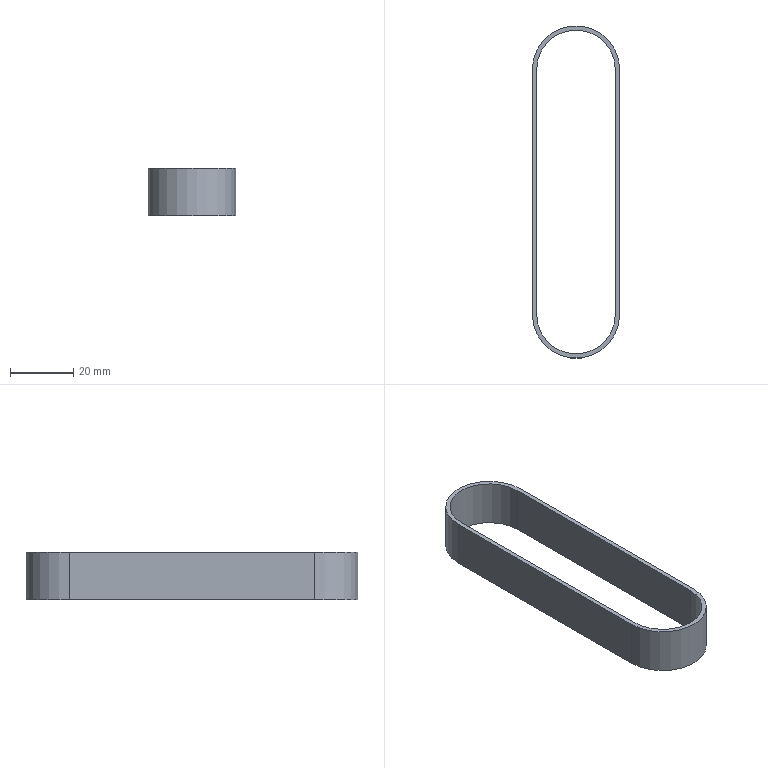Part | NX | features BREP 1 | 1 solid | 10 faces | box 27.59 x 105.06 x 15 mm | volume 4912 mm3 | plane 6 | cylinder 4 | commonest cylinder face diameters 24.83 x2 27.59 x2
STEP:
#1=CARTESIAN_POINT('',(-12.415,38.735,0.));
#2=VERTEX_POINT('',#1);
#3=CARTESIAN_POINT('',(-12.415,-38.735,0.));
#4=VERTEX_POINT('',#3);
#5=CARTESIAN_POINT('',(-12.415,-38.735,0.));
#6=DIRECTION('',(0.,-1.,0.));
#7=VECTOR('',#6,1000.);
#8=LINE('',#5,#7);
#9=EDGE_CURVE('',#2,#4,#8,.T.);
#10=ORIENTED_EDGE('',*,*,#9,.F.);
#11=CARTESIAN_POINT('',(-12.415,38.735,15.));
#12=VERTEX_POINT('',#11);
#13=CARTESIAN_POINT('',(-12.415,38.735,15.));
#14=DIRECTION('',(0.,0.,-1.));
#15=VECTOR('',#14,1000.);
#16=LINE('',#13,#15);
#17=EDGE_CURVE('',#12,#2,#16,.T.);
#18=ORIENTED_EDGE('',*,*,#17,.F.);
#19=CARTESIAN_POINT('',(-12.415,-38.735,15.));
#20=VERTEX_POINT('',#19);
#21=CARTESIAN_POINT('',(-12.415,-38.735,15.));
#22=DIRECTION('',(0.,-1.,0.));
#23=VECTOR('',#22,1000.);
#24=LINE('',#21,#23);
#25=EDGE_CURVE('',#12,#20,#24,.T.);
#26=ORIENTED_EDGE('',*,*,#25,.T.);
#27=CARTESIAN_POINT('',(-12.415,-38.735,15.));
#28=DIRECTION('',(0.,0.,-1.));
#29=VECTOR('',#28,1000.);
#30=LINE('',#27,#29);
#31=EDGE_CURVE('',#20,#4,#30,.T.);
#32=ORIENTED_EDGE('',*,*,#31,.T.);
#33=EDGE_LOOP('',(#10,#18,#26,#32));
#34=FACE_BOUND('',#33,.T.);
#35=CARTESIAN_POINT('',(-12.415,-38.735,15.));
#36=DIRECTION('',(1.,0.,0.));
#37=DIRECTION('',(0.,1.,0.));
#38=AXIS2_PLACEMENT_3D('',#35,#36,#37);
#39=PLANE('',#38);
#40=ADVANCED_FACE('',(#34),#39,.T.);
#41=CARTESIAN_POINT('',(12.415,38.735,0.));
#42=VERTEX_POINT('',#41);
#43=CARTESIAN_POINT('',(0.,38.735,0.));
#44=DIRECTION('',(0.,0.,1.));
#45=DIRECTION('',(1.,0.,0.));
#46=AXIS2_PLACEMENT_3D('',#43,#44,#45);
#47=CIRCLE('',#46,12.415);
#48=EDGE_CURVE('',#42,#2,#47,.T.);
#49=ORIENTED_EDGE('',*,*,#48,.F.);
#50=CARTESIAN_POINT('',(12.415,38.735,15.));
#51=VERTEX_POINT('',#50);
#52=CARTESIAN_POINT('',(12.415,38.735,15.));
#53=DIRECTION('',(0.,0.,-1.));
#54=VECTOR('',#53,1000.);
#55=LINE('',#52,#54);
#56=EDGE_CURVE('',#51,#42,#55,.T.);
#57=ORIENTED_EDGE('',*,*,#56,.F.);
#58=CARTESIAN_POINT('',(0.,38.735,15.));
#59=DIRECTION('',(0.,0.,1.));
#60=DIRECTION('',(1.,0.,0.));
#61=AXIS2_PLACEMENT_3D('',#58,#59,#60);
#62=CIRCLE('',#61,12.415);
#63=EDGE_CURVE('',#51,#12,#62,.T.);
#64=ORIENTED_EDGE('',*,*,#63,.T.);
#65=ORIENTED_EDGE('',*,*,#17,.T.);
#66=EDGE_LOOP('',(#49,#57,#64,#65));
#67=FACE_BOUND('',#66,.T.);
#68=CARTESIAN_POINT('',(0.,38.735,15.));
#69=DIRECTION('',(0.,0.,-1.));
#70=DIRECTION('',(-1.,0.,0.));
#71=AXIS2_PLACEMENT_3D('',#68,#69,#70);
#72=CYLINDRICAL_SURFACE('',#71,12.415);
#73=ADVANCED_FACE('',(#67),#72,.F.);
#74=CARTESIAN_POINT('',(12.415,-38.735,0.));
#75=VERTEX_POINT('',#74);
#76=CARTESIAN_POINT('',(12.415,-38.735,0.));
#77=DIRECTION('',(0.,1.,0.));
#78=VECTOR('',#77,1000.);
#79=LINE('',#76,#78);
#80=EDGE_CURVE('',#75,#42,#79,.T.);
#81=ORIENTED_EDGE('',*,*,#80,.F.);
#82=CARTESIAN_POINT('',(12.415,-38.735,15.));
#83=VERTEX_POINT('',#82);
#84=CARTESIAN_POINT('',(12.415,-38.735,15.));
#85=DIRECTION('',(0.,0.,-1.));
#86=VECTOR('',#85,1000.);
#87=LINE('',#84,#86);
#88=EDGE_CURVE('',#83,#75,#87,.T.);
#89=ORIENTED_EDGE('',*,*,#88,.F.);
#90=CARTESIAN_POINT('',(12.415,-38.735,15.));
#91=DIRECTION('',(0.,1.,0.));
#92=VECTOR('',#91,1000.);
#93=LINE('',#90,#92);
#94=EDGE_CURVE('',#83,#51,#93,.T.);
#95=ORIENTED_EDGE('',*,*,#94,.T.);
#96=ORIENTED_EDGE('',*,*,#56,.T.);
#97=EDGE_LOOP('',(#81,#89,#95,#96));
#98=FACE_BOUND('',#97,.T.);
#99=CARTESIAN_POINT('',(12.415,-38.735,15.));
#100=DIRECTION('',(-1.,0.,0.));
#101=DIRECTION('',(0.,-1.,0.));
#102=AXIS2_PLACEMENT_3D('',#99,#100,#101);
#103=PLANE('',#102);
#104=ADVANCED_FACE('',(#98),#103,.T.);
#105=CARTESIAN_POINT('',(0.,-38.735,0.));
#106=DIRECTION('',(0.,0.,1.));
#107=DIRECTION('',(1.,0.,0.));
#108=AXIS2_PLACEMENT_3D('',#105,#106,#107);
#109=CIRCLE('',#108,12.415);
#110=EDGE_CURVE('',#4,#75,#109,.T.);
#111=ORIENTED_EDGE('',*,*,#110,.F.);
#112=ORIENTED_EDGE('',*,*,#31,.F.);
#113=CARTESIAN_POINT('',(0.,-38.735,15.));
#114=DIRECTION('',(0.,0.,1.));
#115=DIRECTION('',(1.,0.,0.));
#116=AXIS2_PLACEMENT_3D('',#113,#114,#115);
#117=CIRCLE('',#116,12.415);
#118=EDGE_CURVE('',#20,#83,#117,.T.);
#119=ORIENTED_EDGE('',*,*,#118,.T.);
#120=ORIENTED_EDGE('',*,*,#88,.T.);
#121=EDGE_LOOP('',(#111,#112,#119,#120));
#122=FACE_BOUND('',#121,.T.);
#123=CARTESIAN_POINT('',(0.,-38.735,15.));
#124=DIRECTION('',(0.,0.,-1.));
#125=DIRECTION('',(-1.,0.,0.));
#126=AXIS2_PLACEMENT_3D('',#123,#124,#125);
#127=CYLINDRICAL_SURFACE('',#126,12.415);
#128=ADVANCED_FACE('',(#122),#127,.F.);
#129=CARTESIAN_POINT('',(-13.795,38.735,0.));
#130=VERTEX_POINT('',#129);
#131=CARTESIAN_POINT('',(-13.795,-38.735,0.));
#132=VERTEX_POINT('',#131);
#133=CARTESIAN_POINT('',(-13.795,-38.735,0.));
#134=DIRECTION('',(0.,-1.,0.));
#135=VECTOR('',#134,1000.);
#136=LINE('',#133,#135);
#137=EDGE_CURVE('',#130,#132,#136,.T.);
#138=ORIENTED_EDGE('',*,*,#137,.T.);
#139=CARTESIAN_POINT('',(-13.795,-38.735,15.));
#140=VERTEX_POINT('',#139);
#141=CARTESIAN_POINT('',(-13.795,-38.735,15.));
#142=DIRECTION('',(0.,0.,-1.));
#143=VECTOR('',#142,1000.);
#144=LINE('',#141,#143);
#145=EDGE_CURVE('',#140,#132,#144,.T.);
#146=ORIENTED_EDGE('',*,*,#145,.F.);
#147=CARTESIAN_POINT('',(-13.795,38.735,15.));
#148=VERTEX_POINT('',#147);
#149=CARTESIAN_POINT('',(-13.795,-38.735,15.));
#150=DIRECTION('',(0.,-1.,0.));
#151=VECTOR('',#150,1000.);
#152=LINE('',#149,#151);
#153=EDGE_CURVE('',#148,#140,#152,.T.);
#154=ORIENTED_EDGE('',*,*,#153,.F.);
#155=CARTESIAN_POINT('',(-13.795,38.735,15.));
#156=DIRECTION('',(0.,0.,-1.));
#157=VECTOR('',#156,1000.);
#158=LINE('',#155,#157);
#159=EDGE_CURVE('',#148,#130,#158,.T.);
#160=ORIENTED_EDGE('',*,*,#159,.T.);
#161=EDGE_LOOP('',(#138,#146,#154,#160));
#162=FACE_BOUND('',#161,.T.);
#163=CARTESIAN_POINT('',(-13.795,-38.735,15.));
#164=DIRECTION('',(1.,0.,0.));
#165=DIRECTION('',(0.,1.,0.));
#166=AXIS2_PLACEMENT_3D('',#163,#164,#165);
#167=PLANE('',#166);
#168=ADVANCED_FACE('',(#162),#167,.F.);
#169=CARTESIAN_POINT('',(13.795,38.735,0.));
#170=VERTEX_POINT('',#169);
#171=CARTESIAN_POINT('',(0.,38.735,0.));
#172=DIRECTION('',(0.,0.,1.));
#173=DIRECTION('',(1.,0.,0.));
#174=AXIS2_PLACEMENT_3D('',#171,#172,#173);
#175=CIRCLE('',#174,13.795);
#176=EDGE_CURVE('',#170,#130,#175,.T.);
#177=ORIENTED_EDGE('',*,*,#176,.T.);
#178=ORIENTED_EDGE('',*,*,#159,.F.);
#179=CARTESIAN_POINT('',(13.795,38.735,15.));
#180=VERTEX_POINT('',#179);
#181=CARTESIAN_POINT('',(0.,38.735,15.));
#182=DIRECTION('',(0.,0.,1.));
#183=DIRECTION('',(1.,0.,0.));
#184=AXIS2_PLACEMENT_3D('',#181,#182,#183);
#185=CIRCLE('',#184,13.795);
#186=EDGE_CURVE('',#180,#148,#185,.T.);
#187=ORIENTED_EDGE('',*,*,#186,.F.);
#188=CARTESIAN_POINT('',(13.795,38.735,15.));
#189=DIRECTION('',(0.,0.,-1.));
#190=VECTOR('',#189,1000.);
#191=LINE('',#188,#190);
#192=EDGE_CURVE('',#180,#170,#191,.T.);
#193=ORIENTED_EDGE('',*,*,#192,.T.);
#194=EDGE_LOOP('',(#177,#178,#187,#193));
#195=FACE_BOUND('',#194,.T.);
#196=CARTESIAN_POINT('',(0.,38.735,15.));
#197=DIRECTION('',(0.,0.,-1.));
#198=DIRECTION('',(-1.,0.,0.));
#199=AXIS2_PLACEMENT_3D('',#196,#197,#198);
#200=CYLINDRICAL_SURFACE('',#199,13.795);
#201=ADVANCED_FACE('',(#195),#200,.T.);
#202=CARTESIAN_POINT('',(13.795,-38.735,0.));
#203=VERTEX_POINT('',#202);
#204=CARTESIAN_POINT('',(13.795,-38.735,0.));
#205=DIRECTION('',(0.,1.,0.));
#206=VECTOR('',#205,1000.);
#207=LINE('',#204,#206);
#208=EDGE_CURVE('',#203,#170,#207,.T.);
#209=ORIENTED_EDGE('',*,*,#208,.T.);
#210=ORIENTED_EDGE('',*,*,#192,.F.);
#211=CARTESIAN_POINT('',(13.795,-38.735,15.));
#212=VERTEX_POINT('',#211);
#213=CARTESIAN_POINT('',(13.795,-38.735,15.));
#214=DIRECTION('',(0.,1.,0.));
#215=VECTOR('',#214,1000.);
#216=LINE('',#213,#215);
#217=EDGE_CURVE('',#212,#180,#216,.T.);
#218=ORIENTED_EDGE('',*,*,#217,.F.);
#219=CARTESIAN_POINT('',(13.795,-38.735,15.));
#220=DIRECTION('',(0.,0.,-1.));
#221=VECTOR('',#220,1000.);
#222=LINE('',#219,#221);
#223=EDGE_CURVE('',#212,#203,#222,.T.);
#224=ORIENTED_EDGE('',*,*,#223,.T.);
#225=EDGE_LOOP('',(#209,#210,#218,#224));
#226=FACE_BOUND('',#225,.T.);
#227=CARTESIAN_POINT('',(13.795,-38.735,15.));
#228=DIRECTION('',(-1.,0.,0.));
#229=DIRECTION('',(0.,-1.,0.));
#230=AXIS2_PLACEMENT_3D('',#227,#228,#229);
#231=PLANE('',#230);
#232=ADVANCED_FACE('',(#226),#231,.F.);
#233=CARTESIAN_POINT('',(0.,-38.735,0.));
#234=DIRECTION('',(0.,0.,1.));
#235=DIRECTION('',(1.,0.,0.));
#236=AXIS2_PLACEMENT_3D('',#233,#234,#235);
#237=CIRCLE('',#236,13.795);
#238=EDGE_CURVE('',#132,#203,#237,.T.);
#239=ORIENTED_EDGE('',*,*,#238,.T.);
#240=ORIENTED_EDGE('',*,*,#223,.F.);
#241=CARTESIAN_POINT('',(0.,-38.735,15.));
#242=DIRECTION('',(0.,0.,1.));
#243=DIRECTION('',(1.,0.,0.));
#244=AXIS2_PLACEMENT_3D('',#241,#242,#243);
#245=CIRCLE('',#244,13.795);
#246=EDGE_CURVE('',#140,#212,#245,.T.);
#247=ORIENTED_EDGE('',*,*,#246,.F.);
#248=ORIENTED_EDGE('',*,*,#145,.T.);
#249=EDGE_LOOP('',(#239,#240,#247,#248));
#250=FACE_BOUND('',#249,.T.);
#251=CARTESIAN_POINT('',(0.,-38.735,15.));
#252=DIRECTION('',(0.,0.,-1.));
#253=DIRECTION('',(-1.,0.,0.));
#254=AXIS2_PLACEMENT_3D('',#251,#252,#253);
#255=CYLINDRICAL_SURFACE('',#254,13.795);
#256=ADVANCED_FACE('',(#250),#255,.T.);
#257=ORIENTED_EDGE('',*,*,#110,.T.);
#258=ORIENTED_EDGE('',*,*,#80,.T.);
#259=ORIENTED_EDGE('',*,*,#48,.T.);
#260=ORIENTED_EDGE('',*,*,#9,.T.);
#261=EDGE_LOOP('',(#257,#258,#259,#260));
#262=FACE_BOUND('',#261,.T.);
#263=ORIENTED_EDGE('',*,*,#238,.F.);
#264=ORIENTED_EDGE('',*,*,#137,.F.);
#265=ORIENTED_EDGE('',*,*,#176,.F.);
#266=ORIENTED_EDGE('',*,*,#208,.F.);
#267=EDGE_LOOP('',(#263,#264,#265,#266));
#268=FACE_BOUND('',#267,.T.);
#269=CARTESIAN_POINT('',(0.,-38.735,0.));
#270=DIRECTION('',(0.,0.,1.));
#271=DIRECTION('',(1.,0.,0.));
#272=AXIS2_PLACEMENT_3D('',#269,#270,#271);
#273=PLANE('',#272);
#274=ADVANCED_FACE('',(#262,#268),#273,.F.);
#275=ORIENTED_EDGE('',*,*,#94,.F.);
#276=ORIENTED_EDGE('',*,*,#118,.F.);
#277=ORIENTED_EDGE('',*,*,#25,.F.);
#278=ORIENTED_EDGE('',*,*,#63,.F.);
#279=EDGE_LOOP('',(#275,#276,#277,#278));
#280=FACE_BOUND('',#279,.T.);
#281=ORIENTED_EDGE('',*,*,#246,.T.);
#282=ORIENTED_EDGE('',*,*,#217,.T.);
#283=ORIENTED_EDGE('',*,*,#186,.T.);
#284=ORIENTED_EDGE('',*,*,#153,.T.);
#285=EDGE_LOOP('',(#281,#282,#283,#284));
#286=FACE_BOUND('',#285,.T.);
#287=CARTESIAN_POINT('',(0.,-38.735,15.));
#288=DIRECTION('',(0.,0.,1.));
#289=DIRECTION('',(1.,0.,0.));
#290=AXIS2_PLACEMENT_3D('',#287,#288,#289);
#291=PLANE('',#290);
#292=ADVANCED_FACE('',(#280,#286),#291,.T.);
#293=CLOSED_SHELL('',(#40,#73,#104,#128,#168,#201,#232,#256,#274,#292));
#294=MANIFOLD_SOLID_BREP('',#293);
#295=(LENGTH_UNIT()NAMED_UNIT(*)SI_UNIT(.MILLI.,.METRE.));
#296=UNCERTAINTY_MEASURE_WITH_UNIT(LENGTH_MEASURE(0.00001),#295,'','');
#297=(NAMED_UNIT(*)PLANE_ANGLE_UNIT()SI_UNIT($,.RADIAN.));
#298=(NAMED_UNIT(*)SI_UNIT($,.STERADIAN.)SOLID_ANGLE_UNIT());
#299=(GEOMETRIC_REPRESENTATION_CONTEXT(3)GLOBAL_UNCERTAINTY_ASSIGNED_CONTEXT((#296))GLOBAL_UNIT_ASSIGNED_CONTEXT((#295,#297,#298))REPRESENTATION_CONTEXT('',''));
#300=ADVANCED_BREP_SHAPE_REPRESENTATION('',(#294),#299);